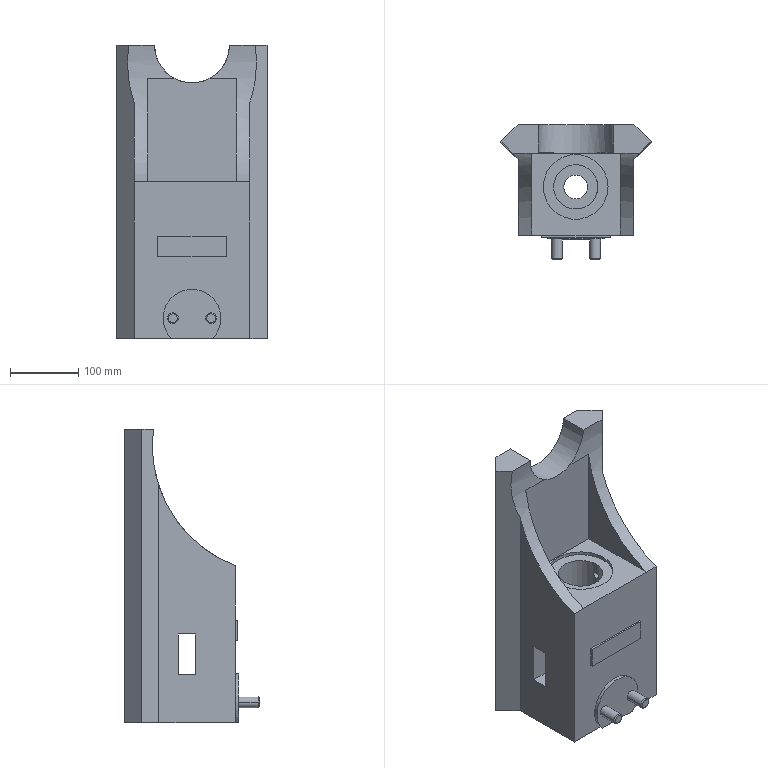Part | Creo | features CURVE 11, CUT 7, PROTRUSION 4, DATUM PLANE 3, CHAMFER 1, COORDINATE SYSTEM 1 | 1 solid | 65 faces | volume 7776005 mm3 | plane 39 | cylinder 22 | cone 4 | commonest cylinder face diameters 16 x8 10 x4 35 x2 65 x2 95 x2 376.095 x2